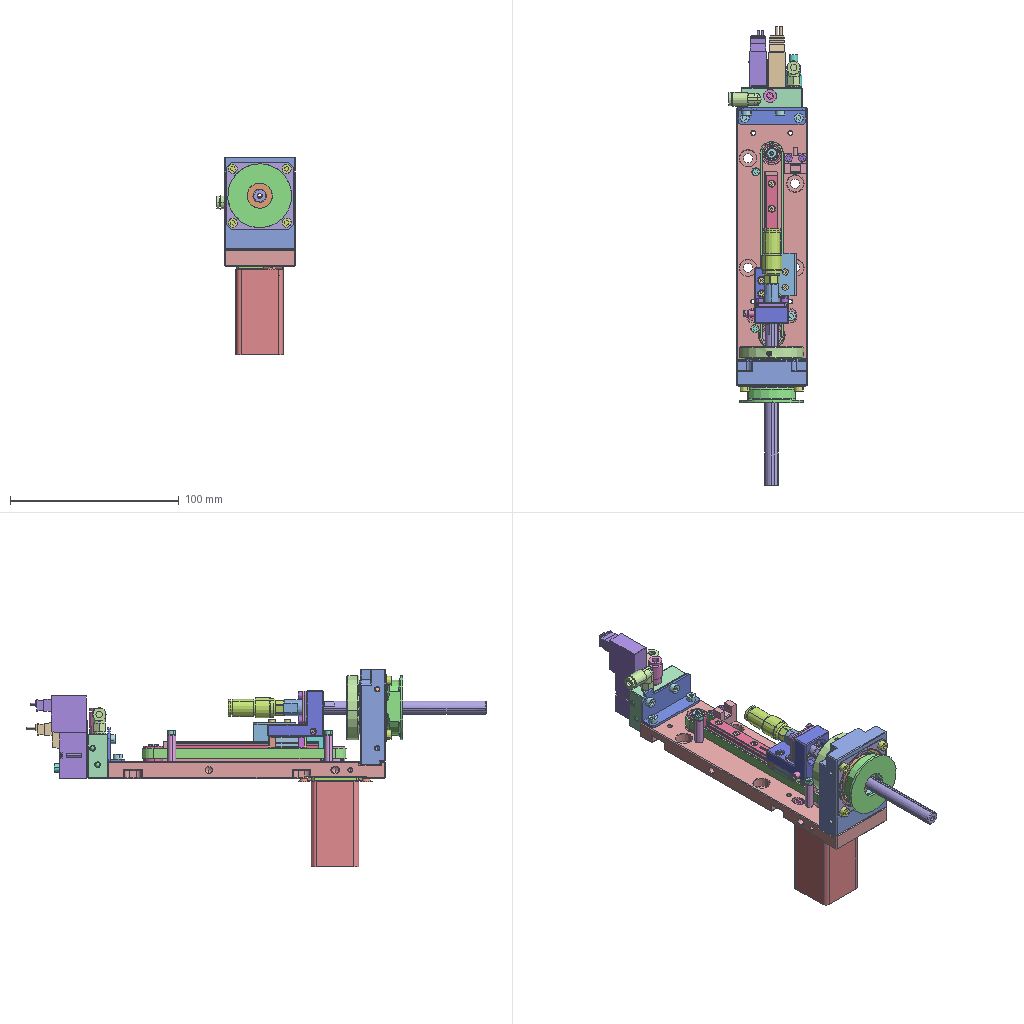Assembly | SolidWorks | 54 different items | 94 placed | box 46 x 273 x 117 mm
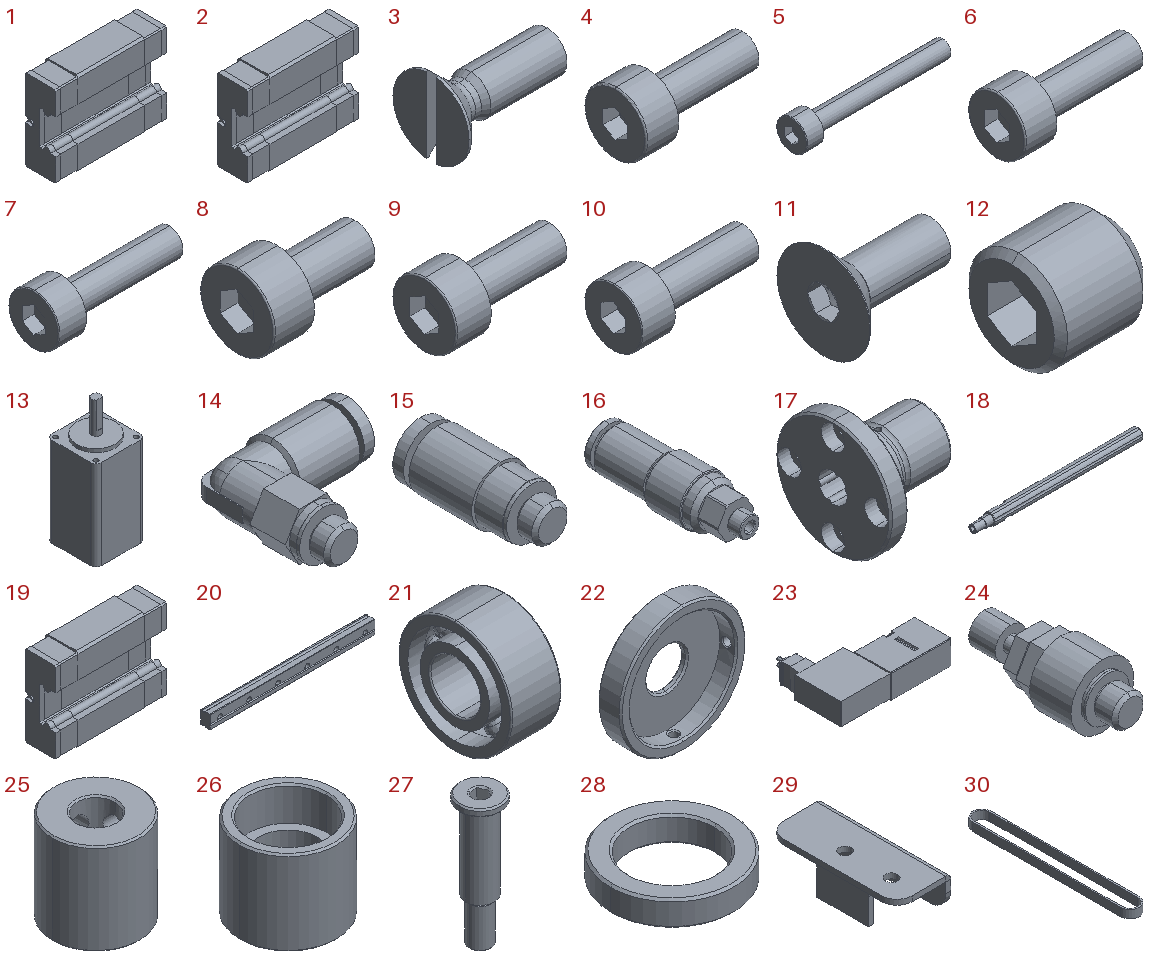Parts list (item | name | quantity | parent item | size | volume | features):
1 | (subassembly) | x1 | - | 22.5 x 6.5 x 17 mm | 1884 mm3 | -
2 | (subassembly) | x1 | in 1 | 22.5 x 6.5 x 17 mm | 1884 mm3 | -
3 | - | x2 | - | 6 x 3.8 x 3.767 mm | 21.27 mm3 | features Chamfer 1, Cut 1, LPattern 1, RevCut 1, Revolution 1
4 | - | x12 | - | 8 x 3.8 x 3.8 mm | 39.383 mm3 | features BlendCut 1, Cut 1, Fillet 1, LPattern 1, RevCut 1, Revolution 1
5 | - | x2 | - | 22.5 x 4.5 x 4.5 mm | 133.887 mm3 | features BlendCut 1, Cut 1, Fillet 1, LPattern 1, RevCut 1, Revolution 1
6 | - | x6 | - | 10.5 x 4.5 x 4.5 mm | 74.982 mm3 | features BlendCut 1, Cut 1, Fillet 1, LPattern 1, RevCut 1, Revolution 1
7 | - | x2 | - | 15 x 5.5 x 5.5 mm | 148.728 mm3 | features BlendCut 1, Cut 1, Fillet 1, LPattern 1, RevCut 1, Revolution 1
8 | - | x4 | - | 9 x 5.5 x 5.5 mm | 106.317 mm3 | features BlendCut 1, Cut 1, Fillet 1, LPattern 1, RevCut 1, Revolution 1
9 | - | x6 | - | 11 x 5.5 x 5.5 mm | 120.454 mm3 | features BlendCut 1, Cut 1, Fillet 1, LPattern 1, RevCut 1, Revolution 1
10 | - | x2 | - | 16 x 7 x 7 mm | 288.227 mm3 | features BlendCut 1, Cut 1, Fillet 1, LPattern 1, RevCut 1, Revolution 1
11 | - | x2 | - | 8 x 6.72 x 6.72 mm | 75.425 mm3 | features RevCut 2, Revolution 2, Cut 1, LPattern 1, RefAxis 1
12 | - | x4 | - | 3 x 3 x 3 mm | 17.39 mm3 | features RevCut 2, Cut 1, LPattern 1, Revolution 1
13 | - | x1 | - | 28.2 x 28.2 x 71 mm | 41213 mm3 | features MBimport 1
14 | - | x2 | - | 19.441 x 18.9 x 8.2 mm | 1067 mm3 | features BaseBody 1
15 | - | x1 | - | 8 x 18.6 x 8 mm | 570.386 mm3 | features BaseBody 1
16 | - | x1 | - | 12 x 36.5 x 12 mm | 2508 mm3 | features ICE 1, Revolution 1
17 | - | x1 | - | 25 x 32 x 32 mm | 6244 mm3 | features BaseBody 1
18 | - | x1 | - | 115 x 8 x 8 mm | 4454 mm3 | features ICE 3, Chamfer 2, BaseBody 1, MoveFace 1
19 | - | x1 | in 2 | 22.5 x 6.5 x 17 mm | 1884 mm3 | features MBimport 1
20 | - | x1 | - | 85 x 4.8 x 7 mm | 2439 mm3 | features BaseBody 1, LPattern 1, MoveFace 1
21 | - | x2 | - | 4 x 9 x 9 mm | 135.884 mm3 | features Revolution 5, CirPattern 2, RevCut 2
22 | - | x1 | - | 38.2 x 7 x 38.2 mm | 3692 mm3 | features 3DProfileFeature 1, HoleWzd 1, ICE 1, Revolution 1
23 | - | x1 | - | 49 x 34.1 x 11.2 mm | 9617 mm3 | features BaseBody 1
24 | - | x1 | - | 10 x 23.3 x 10 mm | 954.231 mm3 | features BaseBody 1
25 | - | x1 | - | 11.46 x 11.46 x 12 mm | 967.917 mm3 | features HoleWzd 2, Revolution 1
26 | - | x1 | - | 11.46 x 11.46 x 10 mm | 442.998 mm3 | features Revolution 1
27 | - | x1 | - | 5.8 x 5.8 x 18.2 mm | 198.341 mm3 | features HoleWzd 1, ICE 1, Revolution 1
28 | - | x1 | - | 5.8 x 5.8 x 1.2 mm | 16.317 mm3 | features Revolution 1
29 | - | x1 | - | 10.5 x 25 x 16 mm | 473.396 mm3 | features ICE 2, Fillet 1, FlatPattern 1, SMBaseFlange 1, SheetMetal 1
30 | - | x1 | - | 13.5 x 121.5 x 6 mm | 1562 mm3 | features Extrusion 1
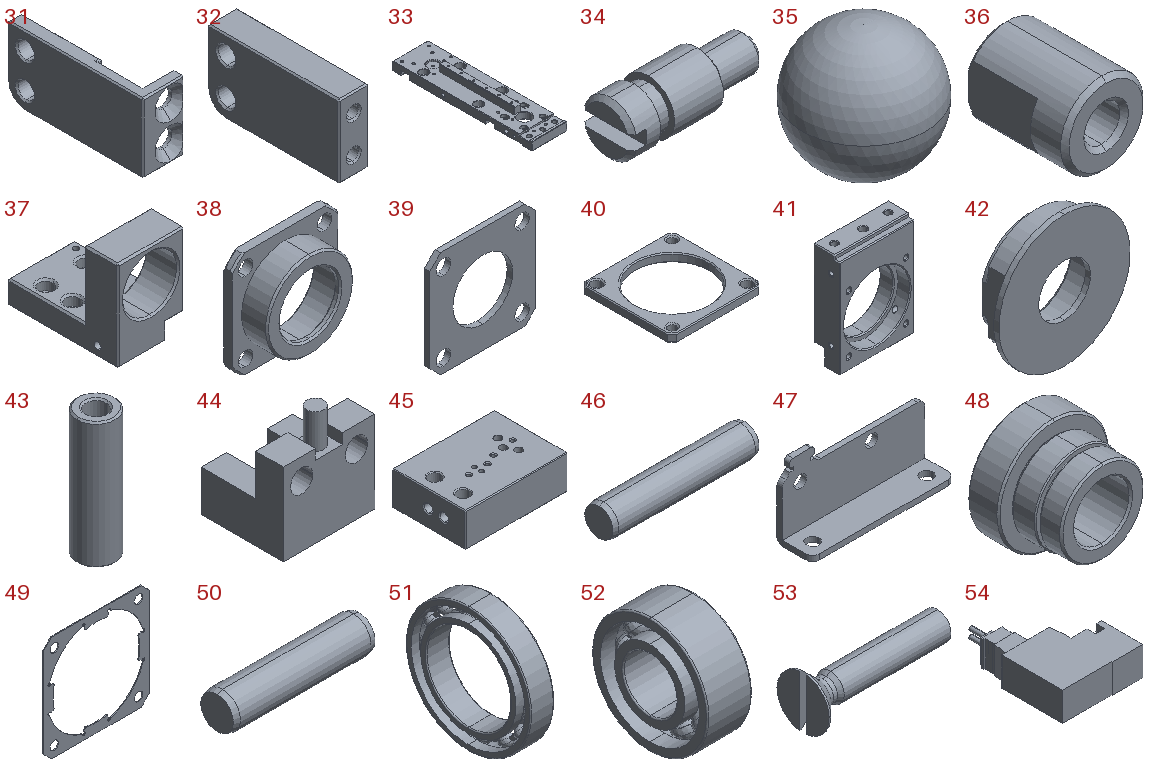31 | - | x1 | - | 6 x 19.5 x 10 mm | 368.969 mm3 | features ICE 3, Chamfer 1, Extrusion 1, Fillet 1, HoleWzd 1
32 | - | x1 | - | 4 x 18 x 10 mm | 638.389 mm3 | features HoleWzd 2, Chamfer 1, Extrusion 1, Fillet 1
33 | - | x1 | - | 42 x 165 x 18 mm | 61836 mm3 | features HoleWzd 13, ICE 13, Chamfer 2, Extrusion 1
34 | - | x1 | - | 10 x 3.8 x 3.8 mm | 81.09 mm3 | features ICE 1, Revolution 1
35 | - | x4 | - | 3.3 x 3.3 x 3.3 mm | 18.817 mm3 | features Revolution 1
36 | - | x1 | - | 9.6 x 12 x 9.6 mm | 642.366 mm3 | features HoleWzd 1, ICE 1, Revolution 1
37 | - | x1 | - | 20 x 33 x 27 mm | 5778 mm3 | features HoleWzd 5, ICE 2, Chamfer 1, Extrusion 1, Fillet 1
38 | - | x1 | - | 19.5 x 6.2 x 19.5 mm | 684.644 mm3 | features ICE 2, Revolution 1
39 | - | x1 | - | 19.5 x 1 x 19.5 mm | 254.315 mm3 | features Extrusion 1, ICE 1
40 | - | x1 | - | 28 x 28 x 2.5 mm | 869.826 mm3 | features Chamfer 1, Extrusion 1, HoleWzd 1, ICE 1
41 | - | x1 | - | 42 x 15 x 57 mm | 19915 mm3 | features HoleWzd 6, ICE 4, Chamfer 1, Extrusion 1
42 | - | x1 | - | 38 x 10 x 38 mm | 4506 mm3 | features HoleWzd 1, ICE 1, Revolution 1
43 | - | x2 | - | 4.8 x 4.8 x 16 mm | 203.651 mm3 | features Revolution 1
44 | - | x1 | - | 13.4 x 12 x 15.5 mm | 1013 mm3 | features ICE 1, MBimport 1, MoveFace 1
45 | - | x1 | - | 36 x 26 x 12 mm | 10025 mm3 | features HoleWzd 14, MoveCopyBody 7, Stock 7, Chamfer 1, Extrusion 1, MoveFace 1
46 | - | x2 | - | 12 x 2.5 x 2.5 mm | 58.578 mm3 | features Revolution 1
47 | - | x1 | - | 40 x 10 x 20 mm | 1427 mm3 | features Fillet 3, ICE 3, FlatPattern 1, SMBaseFlange 1, SheetMetal 1
48 | - | x1 | - | 32 x 23 x 32 mm | 8933 mm3 | features HoleWzd 1, Revolution 1
49 | - | x1 | - | 40 x 0.3 x 40 mm | 162.744 mm3 | features ICE 3, Extrusion 1, Fillet 1
50 | - | x1 | - | 16 x 4 x 4 mm | 199.763 mm3 | features Revolution 1
51 | - | x1 | - | 7 x 37 x 37 mm | 2477 mm3 | features Revolution 5, CirPattern 2, RevCut 2
52 | - | x1 | - | 5 x 13 x 13 mm | 330.95 mm3 | features Revolution 5, CirPattern 2, RevCut 2
53 | - | x2 | - | 10 x 3.8 x 3.767 mm | 33.836 mm3 | features Chamfer 1, Cut 1, LPattern 1, RevCut 1, Revolution 1
54 | - | x1 | - | 27.2 x 36.5 x 9.8 mm | 5427 mm3 | features BaseBody 1
Mates (type | each side: item.copy, entity, surface, feature):
Concentric | 33.1 face cylinder Hole size socket head cap screw type 1 | 41.1 face cylinder M4 Tapped Hole1 | 2 times
Coincident | 33.1 face plane Cut-Extrude2 | 41.1 face plane Boss-Extrude1
Concentric | 33.1 face cylinder Cut-Extrude3 | 40.1 face cylinder Boss-Extrude1
Parallel | 33.1 face plane Boss-Extrude1 | 40.1 face plane Boss-Extrude1
Coincident | 33.1 face plane Cut-Extrude7 | 40.1 face plane Boss-Extrude1
Concentric | 41.1 face cylinder Cut-Extrude2 | 48.1 face cylinder Revolve1
Concentric | 48.1 face cylinder Revolve1 | 51.1 face cylinder Boss-Revolve3
Coincident | 48.1 face plane Revolve1 | 51.1 face plane Boss-Revolve4
Coincident | 41.1 face plane Cut-Extrude1 | 51.1 face plane Boss-Revolve3
Concentric | 48.1 face cylinder Revolve1 | 49.1 face cylinder Cut-Extrude1
Concentric | 41.1 face cylinder M3 Tapped Hole1 | 49.1 face cylinder Cut-Extrude3
Coincident | 41.1 face plane Boss-Extrude1 | 49.1 face plane Boss-Extrude1
Concentric | 48.1 face cylinder Revolve1 | 42.1 face cylinder Revolve1
Coincident | 51.1 face plane Boss-Revolve4 | 42.1 face plane Revolve1
Coincident | 33.1 face plane Cut-Extrude1 | 20.1 face plane MGNR7R85PM_GW202206021814.stp-1/MGR7_temp-1.stp-1-solid1 | 2 times
Concentric | 20.1 face cylinder MGNR7R85PM_GW202206021814.stp-1/MGR7_temp-1.stp-1-solid1 | 19.1 face cylinder MGN7CZ1PM_GW202206021500.stp | 2 times
Concentric | 19.1 face cylinder MGN7CZ1PM_GW202206021500.stp | 37.1 face cylinder Hole size socket head cap screw type 0 | 2 times
Concentric | 37.1 face cylinder M2.5 Tapped Hole2 | 34.1 face cylinder Revolve1
Coincident | 37.1 face plane Boss-Extrude1 | 34.1 face plane Revolve1
Concentric | 37.1 face cylinder M2 Tapped Hole1 | 31.1 face cylinder Cut-Extrude1 | 2 times
Coincident | 37.1 face plane Cut-Extrude4 | 31.1 face plane Boss-Extrude1
Concentric | 31.1 face cylinder Cut-Extrude1 | 32.1 face cylinder Hole size slotted countersunk wood screw type 1 | 2 times
Coincident | 31.1 face plane Boss-Extrude1 | 32.1 face plane Boss-Extrude1
Concentric | 37.1 face cylinder Cut-Extrude1 | 38.1 face cylinder Revolve1
Concentric | 37.1 face cylinder M2.5 Tapped Hole1 | 38.1 face cylinder Cut-Extrude2
Coincident | 37.1 face plane Boss-Extrude1 | 38.1 face plane Revolve1
Concentric | 38.1 face cylinder Revolve1 | 52.1 face cylinder Boss-Revolve3
Coincident | 38.1 face plane Revolve1 | 52.1 face plane Boss-Revolve3
Concentric | 52.1 face cylinder Boss-Revolve4 | 39.1 face cylinder Boss-Extrude1
Coincident | 38.1 face plane Revolve1 | 39.1 face plane Boss-Extrude1
Concentric | 38.1 face cylinder Cut-Extrude2 | 39.1 face cylinder Cut-Extrude1
Coincident | 52.1 face plane Boss-Revolve4 | 36.1 face plane Revolve1
Concentric | 36.1 face cylinder M5 Tapped Hole1 | 16.1 face cylinder Revolve1
Coincident | 36.1 face plane Revolve1 | 16.1 face plane Revolve1
Concentric | 43.1 face cylinder Revolve1 | 5.1 face cylinder Base-Revolve
Coincident | 43.1 face plane Revolve1 | 5.1 face plane Base-Revolve
Coincident | 33.1 face plane Boss-Extrude1 | 43.1 face plane Revolve1
Concentric | 33.1 face cylinder M2.5 Tapped Hole1 | 43.1 face cylinder Revolve1
Concentric | 48.1 face cylinder Revolve1 | 17.1 face cylinder LF_8_FTLF_Cylindar
Concentric | 17.1 face cylinder LF_8_FTLF_Cylindar | 18.1 face cylinder LF_890K_FTLFShaft | 2 times
Concentric | 48.1 face cylinder M3 Tapped Hole1 | 17.1 face cylinder LF_8_FTLF_Cylindar
Coincident | 48.1 face plane Revolve1 | 17.1 face plane LF_8_FTLF_Cylindar
Concentric | 52.1 face cylinder Boss-Revolve4 | 18.1 face cylinder Cut-Extrude2
Coincident | 52.1 face plane Boss-Revolve4 | 18.1 face plane Cut-Extrude1
Concentric | 36.1 face cylinder Revolve1 | 18.1 face cylinder Cut-Extrude2
Concentric | 27.1 face cylinder Revolve1 | 21.1 face cylinder Boss-Revolve3
Concentric | 26.1 face cylinder Revolve1 | 27.1 face cylinder Revolve1
Concentric | 27.1 face cylinder Revolve1 | 21.2 face cylinder Boss-Revolve3
Concentric | 27.1 face cylinder Revolve1 | 28.1 face cylinder Revolve1
Coincident | 27.1 face plane Revolve1 | 21.1 face plane Boss-Revolve4
Coincident | 26.1 face plane Revolve1 | 21.1 face plane Boss-Revolve3
Coincident | 26.1 face plane Revolve1 | 21.2 face plane Boss-Revolve3
Coincident | 21.2 face plane Boss-Revolve4 | 28.1 face plane Revolve1
Concentric | 33.1 face cylinder M3 Tapped Hole2 | 27.1 face cylinder Revolve1
Concentric | 30.1 face cylinder Boss-Extrude1 | 26.1 face cylinder Revolve1
Concentric | 25.1 face cylinder Revolve1 | 30.1 face cylinder Boss-Extrude1
Coincident | 31.1 face plane Boss-Extrude2 | 30.1 face plane Boss-Extrude1
DistanceDim | 20.1 face plane MGNR7R85PM_GW202206021814.stp-1/MGR7_temp-1.stp-1-solid1 | 33.1 face plane Boss-Extrude2
Concentric | 43.2 face cylinder Revolve1 | 5.2 face cylinder Base-Revolve
Coincident | 43.2 face plane Revolve1 | 5.2 face plane Base-Revolve
Coincident | 33.1 face plane Boss-Extrude1 | 43.2 face plane Revolve1
Concentric | 33.1 face cylinder M2.5 Tapped Hole1 | 43.2 face cylinder Revolve1
Coincident | 33.1 face plane Boss-Extrude1 | 45.1 face plane Boss-Extrude1
DistanceDim | 45.1 face plane Boss-Extrude1 | 33.1 face plane Boss-Extrude1
LimitDistanceDim | 20.1 face plane MGNR7R85PM_GW202206021814.stp-1/MGR7_temp-1.stp-1-solid1 | 37.1 face plane Boss-Extrude1
Tangent | 33.1 face plane Cut-Extrude7 | 46.1 face cylinder Base-Revolve
Tangent | 40.1 face plane Boss-Extrude1 | 46.1 face cylinder Base-Revolve
Tangent | 33.1 face plane Cut-Extrude7 | 46.2 face cylinder Base-Revolve
Tangent | 40.1 face plane Boss-Extrude1 | 46.2 face cylinder Base-Revolve
Coincident | 40.1 face plane Boss-Extrude1 | 46.1 face plane Base-Revolve
Concentric | 45.1 face cylinder M3 Tapped Hole1 | 47.1 face cylinder Cut-Extrude1 | 4 times
Coincident | 45.1 face plane Boss-Extrude1 | 47.1 face plane Base-Flange1
Concentric | 45.1 face cylinder M5 Tapped Hole2 | 14.1 face cylinder KQ2L04_M5A
Coincident | 45.1 face plane Boss-Extrude1 | 14.1 face plane KQ2L04_M5A
Parallel | 45.1 face plane Boss-Extrude1 | 14.1 face plane KQ2L04_M5A
Concentric | 45.1 face cylinder M5 Tapped Hole2 | 15.1 face cylinder KQ2S04_M5A
Coincident | 45.1 face plane Boss-Extrude1 | 15.1 face plane KQ2S04_M5A
Concentric | 45.1 face cylinder M5 Tapped Hole1 | 24.1 face cylinder ASN2_M5
Coincident | 45.1 face plane Boss-Extrude1 | 24.1 face plane ASN2_M5
Concentric | 45.1 face cylinder M5 Tapped Hole1 | 14.2 face cylinder KQ2L04_M5A
Coincident | 45.1 face plane Boss-Extrude1 | 14.2 face plane KQ2L04_M5A
Parallel | 45.1 face plane Boss-Extrude1 | 14.2 face plane KQ2L04_M5A
Concentric | 45.1 face cylinder M1.6 Tapped Hole2 | 54.1 face cylinder 10_VQ110_5L_X46 | 2 times
Coincident | 45.1 face plane Boss-Extrude1 | 54.1 face plane 10_VQ110_5L_X46
Concentric | 45.1 face cylinder M1.6 Tapped Hole1 | 23.1 face cylinder VQD1151W_5L | 2 times
Coincident | 45.1 face plane Boss-Extrude1 | 23.1 face plane VQD1151W_5L
Coincident | 33.1 face plane Boss-Extrude1 | 47.1 face plane Base-Flange1
Concentric | 45.1 face cylinder Size mm Dowel PinHole10 | 35.1 face sphere Revolve1
Tangent | 45.1 face plane Boss-Extrude1 | 35.1 face sphere Revolve1
Concentric | 45.1 face cylinder Size mm Dowel PinHole10 | 35.2 face sphere Revolve1
Tangent | 45.1 face plane Boss-Extrude1 | 35.2 face sphere Revolve1
Concentric | 45.1 face cylinder Size mm Dowel PinHole10 | 35.3 face sphere Revolve1
Tangent | 45.1 face plane Boss-Extrude1 | 35.3 face sphere Revolve1
Concentric | 45.1 face cylinder Size mm Dowel Hole5 | 35.4 face sphere Revolve1
Tangent | 45.1 face plane Boss-Extrude1 | 35.4 face sphere Revolve1
Coincident | 33.1 face plane Boss-Extrude1 | 44.1 face plane pm-l25_step.step
Concentric | 37.1 face cylinder M2 Tapped Hole2 | 29.1 face cylinder Cut-Extrude1 | 2 times
Coincident | 37.1 face plane Boss-Extrude1 | 29.1 face plane Base-Flange1
Concentric | 33.1 face cylinder M2.5 Tapped Hole2 | 44.1 face cylinder pm-l25_step.step | 2 times
Coincident | 33.1 face plane Cut-Extrude11 | 27.1 face plane Revolve1
Concentric | 41.1 face cylinder M3 Tapped Hole1 | 8.1 face cylinder Base-Revolve
Coincident | 49.1 face plane Boss-Extrude1 | 8.1 face plane Base-Revolve
Concentric | 41.1 face cylinder M3 Tapped Hole1 | 8.2 face cylinder Base-Revolve
Coincident | 49.1 face plane Boss-Extrude1 | 8.2 face plane Base-Revolve
Concentric | 41.1 face cylinder M3 Tapped Hole1 | 8.3 face cylinder Base-Revolve
Coincident | 49.1 face plane Boss-Extrude1 | 8.3 face plane Base-Revolve
Concentric | 41.1 face cylinder M3 Tapped Hole1 | 8.4 face cylinder Base-Revolve
Coincident | 49.1 face plane Boss-Extrude1 | 8.4 face plane Base-Revolve
Concentric | 32.1 face cylinder Hole size slotted countersunk wood screw type 1 | 53.1 face cylinder Base-Revolve
Coincident | 32.1 face cone Hole size slotted countersunk wood screw type 1 | 53.1 face cone Base-Revolve
Concentric | 32.1 face cylinder Hole size slotted countersunk wood screw type 1 | 53.2 face cylinder Base-Revolve
Coincident | 32.1 face cone Hole size slotted countersunk wood screw type 1 | 53.2 face cone Base-Revolve
Concentric | 31.1 face cylinder Hole size slotted countersunk wood screw type 0 | 3.1 face cylinder Base-Revolve
Coincident | 31.1 face cone Hole size slotted countersunk wood screw type 0 | 3.1 face cone Base-Revolve
Concentric | 31.1 face cylinder Hole size slotted countersunk wood screw type 0 | 3.2 face cylinder Base-Revolve
Coincident | 31.1 face cone Hole size slotted countersunk wood screw type 0 | 3.2 face cone Base-Revolve
Concentric | 33.1 face cylinder M3 Tapped Hole1 | 11.1 face cylinder Revolve1
DistanceDim | 11.1 face plane Revolve1 | 33.1 face plane Cut-Extrude7
Concentric | 33.1 face cylinder M3 Tapped Hole1 | 11.2 face cylinder Revolve1
DistanceDim | 11.2 face plane Revolve1 | 33.1 face plane Cut-Extrude7
Concentric | 41.1 face cylinder Size mm Dowel Hole1 | 50.1 face cylinder Base-Revolve
Coincident | 33.1 face plane Boss-Extrude1 | 50.1 face plane Base-Revolve
Concentric | 33.1 face cylinder Hole size socket head cap screw type 1 | 10.1 face cylinder Base-Revolve
Coincident | 33.1 face plane Hole size socket head cap screw type 1 | 10.1 face plane Base-Revolve
Concentric | 33.1 face cylinder Hole size socket head cap screw type 1 | 10.2 face cylinder Base-Revolve
Coincident | 33.1 face plane Hole size socket head cap screw type 1 | 10.2 face plane Base-Revolve
Coincident | 33.1 face plane Cut-Extrude5 | 7.1 face plane Base-Revolve
Coincident | 33.1 face plane Cut-Extrude5 | 7.2 face plane Base-Revolve
Concentric | 40.1 face cylinder M3 Tapped Hole1 | 9.1 face cylinder Base-Revolve
Coincident | 33.1 face plane Cut-Extrude5 | 9.1 face plane Base-Revolve
Concentric | 40.1 face cylinder M3 Tapped Hole1 | 9.2 face cylinder Base-Revolve
Coincident | 33.1 face plane Cut-Extrude5 | 9.2 face plane Base-Revolve
Concentric | 37.1 face cylinder Hole size socket head cap screw type 0 | 4.1 face cylinder Base-Revolve
Coincident | 37.1 face plane Hole size socket head cap screw type 0 | 4.1 face plane Base-Revolve
Concentric | 37.1 face cylinder Hole size socket head cap screw type 0 | 4.2 face cylinder Base-Revolve
Coincident | 37.1 face plane Hole size socket head cap screw type 0 | 4.2 face plane Base-Revolve
Concentric | 37.1 face cylinder Hole size socket head cap screw type 0 | 4.3 face cylinder Base-Revolve
Coincident | 37.1 face plane Hole size socket head cap screw type 0 | 4.3 face plane Base-Revolve
Concentric | 37.1 face cylinder Hole size socket head cap screw type 0 | 4.4 face cylinder Base-Revolve
Coincident | 37.1 face plane Hole size socket head cap screw type 0 | 4.4 face plane Base-Revolve
Concentric | 20.1 face cylinder MGNR7R85PM_GW202206021814.stp-1/MGR7_temp-1.stp-1-solid1 | 4.5 face cylinder Base-Revolve
Coincident | 20.1 face plane MGNR7R85PM_GW202206021814.stp-1/MGR7_temp-1.stp-1-solid1 | 4.5 face plane Base-Revolve
Concentric | 20.1 face cylinder MGNR7R85PM_GW202206021814.stp-1/MGR7_temp-1.stp-1-solid1 | 4.6 face cylinder Base-Revolve
Coincident | 20.1 face plane MGNR7R85PM_GW202206021814.stp-1/MGR7_temp-1.stp-1-solid1 | 4.6 face plane Base-Revolve
Concentric | 20.1 face cylinder LPattern1 | 4.7 face cylinder Base-Revolve
Coincident | 20.1 face plane LPattern1 | 4.7 face plane Base-Revolve
Concentric | 20.1 face cylinder LPattern1 | 4.8 face cylinder Base-Revolve
Coincident | 20.1 face plane LPattern1 | 4.8 face plane Base-Revolve
Concentric | 20.1 face cylinder MGNR7R85PM_GW202206021814.stp-1/MGR7_temp-1.stp-1-solid1 | 4.9 face cylinder Base-Revolve
Coincident | 20.1 face plane MGNR7R85PM_GW202206021814.stp-1/MGR7_temp-1.stp-1-solid1 | 4.9 face plane Base-Revolve
Concentric | 20.1 face cylinder MGNR7R85PM_GW202206021814.stp-1/MGR7_temp-1.stp-1-solid1 | 4.10 face cylinder Base-Revolve
Coincident | 20.1 face plane MGNR7R85PM_GW202206021814.stp-1/MGR7_temp-1.stp-1-solid1 | 4.10 face plane Base-Revolve
Concentric | 37.1 face cylinder M2 Tapped Hole2 | 4.11 face cylinder Base-Revolve
Coincident | 29.1 face plane Base-Flange1 | 4.11 face plane Base-Revolve
Concentric | 37.1 face cylinder M2 Tapped Hole2 | 4.12 face cylinder Base-Revolve
Coincident | 29.1 face plane Base-Flange1 | 4.12 face plane Base-Revolve
Concentric | 33.1 face cylinder M2.5 Tapped Hole2 | 6.1 face cylinder Base-Revolve
Coincident | 44.1 face plane pm-l25_step.step | 6.1 face plane Base-Revolve
Concentric | 33.1 face cylinder M2.5 Tapped Hole2 | 6.2 face cylinder Base-Revolve
Coincident | 44.1 face plane pm-l25_step.step | 6.2 face plane Base-Revolve
Concentric | 33.1 face cylinder M3 Tapped Hole3 | 9.3 face cylinder Base-Revolve
Coincident | 47.1 face plane Base-Flange1 | 9.3 face plane Base-Revolve
Concentric | 47.1 face cylinder Cut-Extrude1 | 9.4 face cylinder Base-Revolve
Coincident | 47.1 face plane Base-Flange1 | 9.4 face plane Base-Revolve
Concentric | 47.1 face cylinder Cut-Extrude1 | 9.5 face cylinder Base-Revolve
Coincident | 47.1 face plane Base-Flange1 | 9.5 face plane Base-Revolve
Concentric | 47.1 face cylinder Cut-Extrude2 | 9.6 face cylinder Base-Revolve
Coincident | 47.1 face plane Base-Flange1 | 9.6 face plane Base-Revolve
Concentric | 39.1 face cylinder Cut-Extrude1 | 6.3 face cylinder Base-Revolve
Coincident | 39.1 face plane Boss-Extrude1 | 6.3 face plane Base-Revolve
Concentric | 39.1 face cylinder Cut-Extrude1 | 6.4 face cylinder Base-Revolve
Coincident | 39.1 face plane Boss-Extrude1 | 6.4 face plane Base-Revolve
Concentric | 39.1 face cylinder Cut-Extrude1 | 6.5 face cylinder Base-Revolve
Coincident | 39.1 face plane Boss-Extrude1 | 6.5 face plane Base-Revolve
Concentric | 39.1 face cylinder Cut-Extrude1 | 6.6 face cylinder Base-Revolve
Coincident | 39.1 face plane Boss-Extrude1 | 6.6 face plane Base-Revolve
Concentric | 22.1 face cylinder M3 Tapped Hole1 | 12.1 face cylinder Base-Revolve
Tangent | 22.1 face cylinder Revolve1 | 12.1 face plane Base-Revolve
Concentric | 22.1 face cylinder Revolve1 | 17.1 face cylinder LF_8_FTLF_Cylindar
Coincident | 22.1 face plane Revolve1 | 17.1 face plane LF_8_FTLF_Cylindar
Concentric | 22.1 face cylinder M3 Tapped Hole1 | 12.2 face cylinder Base-Revolve
Tangent | 22.1 face cylinder Revolve1 | 12.2 face plane Base-Revolve
Concentric | 25.1 face cylinder M3 Tapped Hole2 | 12.3 face cylinder Base-Revolve
Tangent | 25.1 face cylinder Revolve1 | 12.3 face plane Base-Revolve
Concentric | 25.1 face cylinder M3 Tapped Hole1 | 12.4 face cylinder Base-Revolve
Tangent | 25.1 face cylinder Revolve1 | 12.4 face plane Base-Revolve
Concentric | 33.1 face cylinder Cut-Extrude3 | 13.1 face cylinder 28CM013.STEP
Concentric | 40.1 face cylinder Cut-Extrude1 | 7.1 face cylinder Base-Revolve
Concentric | 40.1 face cylinder Cut-Extrude1 | 7.2 face cylinder Base-Revolve
Concentric | 7.2 face cylinder Base-Revolve | 13.1 face cylinder 28CM013.STEP
Coincident | 40.1 face plane Boss-Extrude1 | 13.1 face plane 28CM013.STEP
Coincident | 33.1 face plane Cut-Extrude10 | 46.2 face plane Base-Revolve